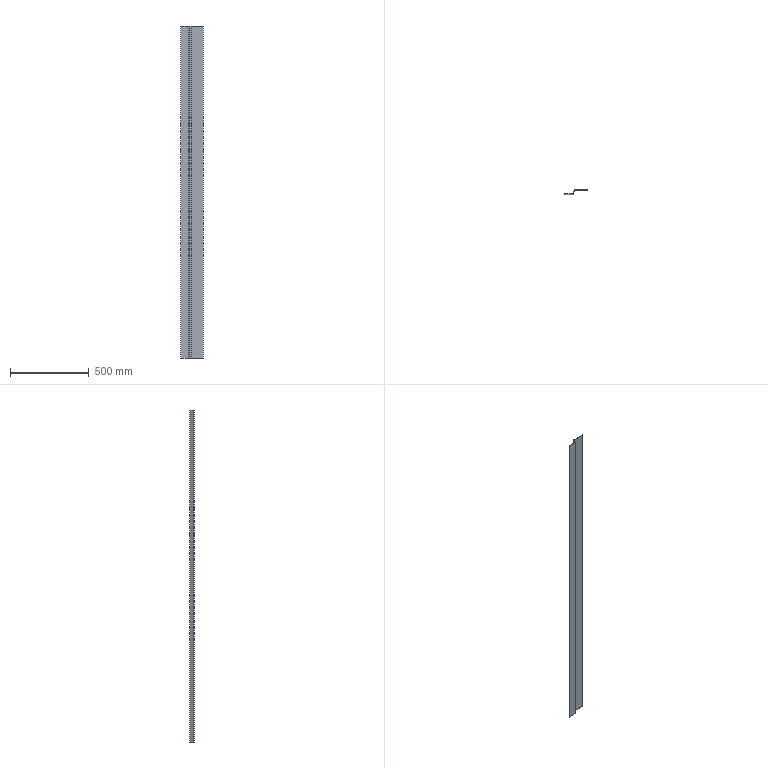Part | STEP file | 750038163 | 1 solid | 14 faces | box 144 x 29 x 2114 mm | volume 1005017 mm3 | plane 10 | cylinder 4 | commonest cylinder face diameters 6 x2 12 x2
STEP:
#1=CARTESIAN_POINT('',(-76.416,0.,1057.));
#2=VERTEX_POINT('',#1);
#3=CARTESIAN_POINT('',(0.,0.,1057.));
#4=VERTEX_POINT('',#3);
#5=CARTESIAN_POINT('',(-80.,0.,1057.));
#6=DIRECTION('',(1.,0.,0.));
#7=VECTOR('',#6,1000.);
#8=LINE('',#5,#7);
#9=EDGE_CURVE('',#2,#4,#8,.T.);
#10=ORIENTED_EDGE('',*,*,#9,.T.);
#11=CARTESIAN_POINT('',(0.,0.,-1057.));
#12=VERTEX_POINT('',#11);
#13=CARTESIAN_POINT('',(0.,0.,1057.));
#14=DIRECTION('',(0.,0.,-1.));
#15=VECTOR('',#14,1000.);
#16=LINE('',#13,#15);
#17=EDGE_CURVE('',#4,#12,#16,.T.);
#18=ORIENTED_EDGE('',*,*,#17,.T.);
#19=CARTESIAN_POINT('',(-76.416,0.,-1057.));
#20=VERTEX_POINT('',#19);
#21=CARTESIAN_POINT('',(-80.,0.,-1057.));
#22=DIRECTION('',(-1.,0.,0.));
#23=VECTOR('',#22,1000.);
#24=LINE('',#21,#23);
#25=EDGE_CURVE('',#12,#20,#24,.T.);
#26=ORIENTED_EDGE('',*,*,#25,.T.);
#27=CARTESIAN_POINT('',(-76.416,0.,1057.));
#28=DIRECTION('',(0.,0.,1.));
#29=VECTOR('',#28,1000.);
#30=LINE('',#27,#29);
#31=EDGE_CURVE('',#20,#2,#30,.T.);
#32=ORIENTED_EDGE('',*,*,#31,.T.);
#33=EDGE_LOOP('',(#10,#18,#26,#32));
#34=FACE_OUTER_BOUND('',#33,.T.);
#35=CARTESIAN_POINT('',(-80.,0.,1057.));
#36=DIRECTION('',(0.,1.,0.));
#37=DIRECTION('',(-1.,0.,0.));
#38=AXIS2_PLACEMENT_3D('',#35,#36,#37);
#39=PLANE('',#38);
#40=ADVANCED_FACE('',(#34),#39,.T.);
#41=CARTESIAN_POINT('',(0.,-3.,-1057.));
#42=VERTEX_POINT('',#41);
#43=CARTESIAN_POINT('',(0.,0.,-1057.));
#44=DIRECTION('',(0.,1.,0.));
#45=VECTOR('',#44,1000.);
#46=LINE('',#43,#45);
#47=EDGE_CURVE('',#42,#12,#46,.T.);
#48=ORIENTED_EDGE('',*,*,#47,.T.);
#49=ORIENTED_EDGE('',*,*,#17,.F.);
#50=CARTESIAN_POINT('',(0.,-3.,1057.));
#51=VERTEX_POINT('',#50);
#52=CARTESIAN_POINT('',(0.,0.,1057.));
#53=DIRECTION('',(0.,-1.,0.));
#54=VECTOR('',#53,1000.);
#55=LINE('',#52,#54);
#56=EDGE_CURVE('',#4,#51,#55,.T.);
#57=ORIENTED_EDGE('',*,*,#56,.T.);
#58=CARTESIAN_POINT('',(0.,-3.,1057.));
#59=DIRECTION('',(0.,0.,-1.));
#60=VECTOR('',#59,1000.);
#61=LINE('',#58,#60);
#62=EDGE_CURVE('',#51,#42,#61,.T.);
#63=ORIENTED_EDGE('',*,*,#62,.T.);
#64=EDGE_LOOP('',(#48,#49,#57,#63));
#65=FACE_OUTER_BOUND('',#64,.T.);
#66=CARTESIAN_POINT('',(0.,0.,1057.));
#67=DIRECTION('',(1.,0.,0.));
#68=DIRECTION('',(0.,1.,0.));
#69=AXIS2_PLACEMENT_3D('',#66,#67,#68);
#70=PLANE('',#69);
#71=ADVANCED_FACE('',(#65),#70,.T.);
#72=CARTESIAN_POINT('',(-76.416,-3.,1057.));
#73=VERTEX_POINT('',#72);
#74=CARTESIAN_POINT('',(-80.,-3.,1057.));
#75=DIRECTION('',(1.,0.,0.));
#76=VECTOR('',#75,1000.);
#77=LINE('',#74,#76);
#78=EDGE_CURVE('',#73,#51,#77,.T.);
#79=ORIENTED_EDGE('',*,*,#78,.T.);
#80=ORIENTED_EDGE('',*,*,#56,.F.);
#81=ORIENTED_EDGE('',*,*,#9,.F.);
#82=CARTESIAN_POINT('',(-81.699,-3.155,1057.));
#83=VERTEX_POINT('',#82);
#84=CARTESIAN_POINT('',(-76.416,-6.,1057.));
#85=DIRECTION('',(0.,0.,1.));
#86=DIRECTION('',(-1.,0.,0.));
#87=AXIS2_PLACEMENT_3D('',#84,#85,#86);
#88=CIRCLE('',#87,6.);
#89=EDGE_CURVE('',#2,#83,#88,.T.);
#90=ORIENTED_EDGE('',*,*,#89,.T.);
#91=CARTESIAN_POINT('',(-93.15,-24.422,1057.));
#92=VERTEX_POINT('',#91);
#93=CARTESIAN_POINT('',(-81.699,-3.155,1057.));
#94=DIRECTION('',(-0.4741,-0.8805,0.));
#95=VECTOR('',#94,1000.);
#96=LINE('',#93,#95);
#97=EDGE_CURVE('',#83,#92,#96,.T.);
#98=ORIENTED_EDGE('',*,*,#97,.T.);
#99=CARTESIAN_POINT('',(-95.792,-26.,1057.));
#100=VERTEX_POINT('',#99);
#101=CARTESIAN_POINT('',(-95.792,-23.,1057.));
#102=DIRECTION('',(0.,0.,-1.));
#103=DIRECTION('',(-1.,0.,0.));
#104=AXIS2_PLACEMENT_3D('',#101,#102,#103);
#105=CIRCLE('',#104,3.);
#106=EDGE_CURVE('',#92,#100,#105,.T.);
#107=ORIENTED_EDGE('',*,*,#106,.T.);
#108=CARTESIAN_POINT('',(-144.,-26.,1057.));
#109=VERTEX_POINT('',#108);
#110=CARTESIAN_POINT('',(-80.,-26.,1057.));
#111=DIRECTION('',(-1.,0.,0.));
#112=VECTOR('',#111,1000.);
#113=LINE('',#110,#112);
#114=EDGE_CURVE('',#100,#109,#113,.T.);
#115=ORIENTED_EDGE('',*,*,#114,.T.);
#116=CARTESIAN_POINT('',(-144.,-29.,1057.));
#117=VERTEX_POINT('',#116);
#118=CARTESIAN_POINT('',(-144.,0.,1057.));
#119=DIRECTION('',(0.,-1.,0.));
#120=VECTOR('',#119,1000.);
#121=LINE('',#118,#120);
#122=EDGE_CURVE('',#109,#117,#121,.T.);
#123=ORIENTED_EDGE('',*,*,#122,.T.);
#124=CARTESIAN_POINT('',(-95.792,-29.,1057.));
#125=VERTEX_POINT('',#124);
#126=CARTESIAN_POINT('',(-80.,-29.,1057.));
#127=DIRECTION('',(1.,0.,0.));
#128=VECTOR('',#127,1000.);
#129=LINE('',#126,#128);
#130=EDGE_CURVE('',#117,#125,#129,.T.);
#131=ORIENTED_EDGE('',*,*,#130,.T.);
#132=CARTESIAN_POINT('',(-90.509,-25.845,1057.));
#133=VERTEX_POINT('',#132);
#134=CARTESIAN_POINT('',(-95.792,-23.,1057.));
#135=DIRECTION('',(0.,0.,1.));
#136=DIRECTION('',(-1.,0.,0.));
#137=AXIS2_PLACEMENT_3D('',#134,#135,#136);
#138=CIRCLE('',#137,6.);
#139=EDGE_CURVE('',#125,#133,#138,.T.);
#140=ORIENTED_EDGE('',*,*,#139,.T.);
#141=CARTESIAN_POINT('',(-79.058,-4.578,1057.));
#142=VERTEX_POINT('',#141);
#143=CARTESIAN_POINT('',(-90.509,-25.845,1057.));
#144=DIRECTION('',(0.4741,0.8805,0.));
#145=VECTOR('',#144,1000.);
#146=LINE('',#143,#145);
#147=EDGE_CURVE('',#133,#142,#146,.T.);
#148=ORIENTED_EDGE('',*,*,#147,.T.);
#149=CARTESIAN_POINT('',(-76.416,-6.,1057.));
#150=DIRECTION('',(0.,0.,-1.));
#151=DIRECTION('',(-1.,0.,0.));
#152=AXIS2_PLACEMENT_3D('',#149,#150,#151);
#153=CIRCLE('',#152,3.);
#154=EDGE_CURVE('',#142,#73,#153,.T.);
#155=ORIENTED_EDGE('',*,*,#154,.T.);
#156=EDGE_LOOP('',(#79,#80,#81,#90,#98,#107,#115,#123,#131,#140,#148,#155));
#157=FACE_OUTER_BOUND('',#156,.T.);
#158=CARTESIAN_POINT('',(-80.,0.,1057.));
#159=DIRECTION('',(0.,0.,1.));
#160=DIRECTION('',(1.,0.,0.));
#161=AXIS2_PLACEMENT_3D('',#158,#159,#160);
#162=PLANE('',#161);
#163=ADVANCED_FACE('',(#157),#162,.T.);
#164=ORIENTED_EDGE('',*,*,#89,.F.);
#165=ORIENTED_EDGE('',*,*,#31,.F.);
#166=CARTESIAN_POINT('',(-81.699,-3.155,-1057.));
#167=VERTEX_POINT('',#166);
#168=CARTESIAN_POINT('',(-76.416,-6.,-1057.));
#169=DIRECTION('',(0.,0.,1.));
#170=DIRECTION('',(-1.,0.,0.));
#171=AXIS2_PLACEMENT_3D('',#168,#169,#170);
#172=CIRCLE('',#171,6.);
#173=EDGE_CURVE('',#20,#167,#172,.T.);
#174=ORIENTED_EDGE('',*,*,#173,.T.);
#175=CARTESIAN_POINT('',(-81.699,-3.155,1057.));
#176=DIRECTION('',(0.,0.,1.));
#177=VECTOR('',#176,1000.);
#178=LINE('',#175,#177);
#179=EDGE_CURVE('',#167,#83,#178,.T.);
#180=ORIENTED_EDGE('',*,*,#179,.T.);
#181=EDGE_LOOP('',(#164,#165,#174,#180));
#182=FACE_OUTER_BOUND('',#181,.T.);
#183=CARTESIAN_POINT('',(-76.416,-6.,1057.));
#184=DIRECTION('',(0.,0.,-1.));
#185=DIRECTION('',(-1.,0.,0.));
#186=AXIS2_PLACEMENT_3D('',#183,#184,#185);
#187=CYLINDRICAL_SURFACE('',#186,6.);
#188=ADVANCED_FACE('',(#182),#187,.T.);
#189=CARTESIAN_POINT('',(-93.15,-24.422,-1057.));
#190=VERTEX_POINT('',#189);
#191=CARTESIAN_POINT('',(-95.792,-26.,-1057.));
#192=VERTEX_POINT('',#191);
#193=CARTESIAN_POINT('',(-95.792,-23.,-1057.));
#194=DIRECTION('',(0.,0.,-1.));
#195=DIRECTION('',(-1.,0.,0.));
#196=AXIS2_PLACEMENT_3D('',#193,#194,#195);
#197=CIRCLE('',#196,3.);
#198=EDGE_CURVE('',#190,#192,#197,.T.);
#199=ORIENTED_EDGE('',*,*,#198,.F.);
#200=CARTESIAN_POINT('',(-81.699,-3.155,-1057.));
#201=DIRECTION('',(-0.4741,-0.8805,0.));
#202=VECTOR('',#201,1000.);
#203=LINE('',#200,#202);
#204=EDGE_CURVE('',#167,#190,#203,.T.);
#205=ORIENTED_EDGE('',*,*,#204,.F.);
#206=ORIENTED_EDGE('',*,*,#173,.F.);
#207=ORIENTED_EDGE('',*,*,#25,.F.);
#208=ORIENTED_EDGE('',*,*,#47,.F.);
#209=CARTESIAN_POINT('',(-76.416,-3.,-1057.));
#210=VERTEX_POINT('',#209);
#211=CARTESIAN_POINT('',(-144.,-3.,-1057.));
#212=DIRECTION('',(1.,0.,0.));
#213=VECTOR('',#212,1000.);
#214=LINE('',#211,#213);
#215=EDGE_CURVE('',#210,#42,#214,.T.);
#216=ORIENTED_EDGE('',*,*,#215,.F.);
#217=CARTESIAN_POINT('',(-79.058,-4.578,-1057.));
#218=VERTEX_POINT('',#217);
#219=CARTESIAN_POINT('',(-76.416,-6.,-1057.));
#220=DIRECTION('',(0.,0.,-1.));
#221=DIRECTION('',(-1.,0.,0.));
#222=AXIS2_PLACEMENT_3D('',#219,#220,#221);
#223=CIRCLE('',#222,3.);
#224=EDGE_CURVE('',#218,#210,#223,.T.);
#225=ORIENTED_EDGE('',*,*,#224,.F.);
#226=CARTESIAN_POINT('',(-90.509,-25.845,-1057.));
#227=VERTEX_POINT('',#226);
#228=CARTESIAN_POINT('',(-90.509,-25.845,-1057.));
#229=DIRECTION('',(0.4741,0.8805,0.));
#230=VECTOR('',#229,1000.);
#231=LINE('',#228,#230);
#232=EDGE_CURVE('',#227,#218,#231,.T.);
#233=ORIENTED_EDGE('',*,*,#232,.F.);
#234=CARTESIAN_POINT('',(-95.792,-29.,-1057.));
#235=VERTEX_POINT('',#234);
#236=CARTESIAN_POINT('',(-95.792,-23.,-1057.));
#237=DIRECTION('',(0.,0.,1.));
#238=DIRECTION('',(-1.,0.,0.));
#239=AXIS2_PLACEMENT_3D('',#236,#237,#238);
#240=CIRCLE('',#239,6.);
#241=EDGE_CURVE('',#235,#227,#240,.T.);
#242=ORIENTED_EDGE('',*,*,#241,.F.);
#243=CARTESIAN_POINT('',(-144.,-29.,-1057.));
#244=VERTEX_POINT('',#243);
#245=CARTESIAN_POINT('',(-144.,-29.,-1057.));
#246=DIRECTION('',(1.,0.,0.));
#247=VECTOR('',#246,1000.);
#248=LINE('',#245,#247);
#249=EDGE_CURVE('',#244,#235,#248,.T.);
#250=ORIENTED_EDGE('',*,*,#249,.F.);
#251=CARTESIAN_POINT('',(-144.,-26.,-1057.));
#252=VERTEX_POINT('',#251);
#253=CARTESIAN_POINT('',(-144.,-26.,-1057.));
#254=DIRECTION('',(0.,-1.,0.));
#255=VECTOR('',#254,1000.);
#256=LINE('',#253,#255);
#257=EDGE_CURVE('',#252,#244,#256,.T.);
#258=ORIENTED_EDGE('',*,*,#257,.F.);
#259=CARTESIAN_POINT('',(-144.,-26.,-1057.));
#260=DIRECTION('',(-1.,0.,0.));
#261=VECTOR('',#260,1000.);
#262=LINE('',#259,#261);
#263=EDGE_CURVE('',#192,#252,#262,.T.);
#264=ORIENTED_EDGE('',*,*,#263,.F.);
#265=EDGE_LOOP('',(#199,#205,#206,#207,#208,#216,#225,#233,#242,#250,#258,#264));
#266=FACE_OUTER_BOUND('',#265,.T.);
#267=CARTESIAN_POINT('',(-144.,-26.,-1057.));
#268=DIRECTION('',(0.,0.,1.));
#269=DIRECTION('',(1.,0.,0.));
#270=AXIS2_PLACEMENT_3D('',#267,#268,#269);
#271=PLANE('',#270);
#272=ADVANCED_FACE('',(#266),#271,.F.);
#273=ORIENTED_EDGE('',*,*,#62,.F.);
#274=ORIENTED_EDGE('',*,*,#78,.F.);
#275=CARTESIAN_POINT('',(-76.416,-3.,1057.));
#276=DIRECTION('',(0.,0.,1.));
#277=VECTOR('',#276,1000.);
#278=LINE('',#275,#277);
#279=EDGE_CURVE('',#210,#73,#278,.T.);
#280=ORIENTED_EDGE('',*,*,#279,.F.);
#281=ORIENTED_EDGE('',*,*,#215,.T.);
#282=EDGE_LOOP('',(#273,#274,#280,#281));
#283=FACE_OUTER_BOUND('',#282,.T.);
#284=CARTESIAN_POINT('',(-80.,-3.,1057.));
#285=DIRECTION('',(0.,1.,0.));
#286=DIRECTION('',(-1.,0.,0.));
#287=AXIS2_PLACEMENT_3D('',#284,#285,#286);
#288=PLANE('',#287);
#289=ADVANCED_FACE('',(#283),#288,.F.);
#290=ORIENTED_EDGE('',*,*,#279,.T.);
#291=ORIENTED_EDGE('',*,*,#154,.F.);
#292=CARTESIAN_POINT('',(-79.058,-4.578,1057.));
#293=DIRECTION('',(0.,0.,1.));
#294=VECTOR('',#293,1000.);
#295=LINE('',#292,#294);
#296=EDGE_CURVE('',#218,#142,#295,.T.);
#297=ORIENTED_EDGE('',*,*,#296,.F.);
#298=ORIENTED_EDGE('',*,*,#224,.T.);
#299=EDGE_LOOP('',(#290,#291,#297,#298));
#300=FACE_OUTER_BOUND('',#299,.T.);
#301=CARTESIAN_POINT('',(-76.416,-6.,1057.));
#302=DIRECTION('',(0.,0.,-1.));
#303=DIRECTION('',(-1.,0.,0.));
#304=AXIS2_PLACEMENT_3D('',#301,#302,#303);
#305=CYLINDRICAL_SURFACE('',#304,3.);
#306=ADVANCED_FACE('',(#300),#305,.F.);
#307=ORIENTED_EDGE('',*,*,#296,.T.);
#308=ORIENTED_EDGE('',*,*,#147,.F.);
#309=CARTESIAN_POINT('',(-90.509,-25.845,1057.));
#310=DIRECTION('',(0.,0.,1.));
#311=VECTOR('',#310,1000.);
#312=LINE('',#309,#311);
#313=EDGE_CURVE('',#227,#133,#312,.T.);
#314=ORIENTED_EDGE('',*,*,#313,.F.);
#315=ORIENTED_EDGE('',*,*,#232,.T.);
#316=EDGE_LOOP('',(#307,#308,#314,#315));
#317=FACE_OUTER_BOUND('',#316,.T.);
#318=CARTESIAN_POINT('',(-91.359,-27.422,1057.));
#319=DIRECTION('',(-0.8805,0.4741,0.));
#320=DIRECTION('',(-0.4741,-0.8805,0.));
#321=AXIS2_PLACEMENT_3D('',#318,#319,#320);
#322=PLANE('',#321);
#323=ADVANCED_FACE('',(#317),#322,.F.);
#324=ORIENTED_EDGE('',*,*,#139,.F.);
#325=CARTESIAN_POINT('',(-95.792,-29.,1057.));
#326=DIRECTION('',(0.,0.,-1.));
#327=VECTOR('',#326,1000.);
#328=LINE('',#325,#327);
#329=EDGE_CURVE('',#125,#235,#328,.T.);
#330=ORIENTED_EDGE('',*,*,#329,.T.);
#331=ORIENTED_EDGE('',*,*,#241,.T.);
#332=ORIENTED_EDGE('',*,*,#313,.T.);
#333=EDGE_LOOP('',(#324,#330,#331,#332));
#334=FACE_OUTER_BOUND('',#333,.T.);
#335=CARTESIAN_POINT('',(-95.792,-23.,1057.));
#336=DIRECTION('',(0.,0.,-1.));
#337=DIRECTION('',(-1.,0.,0.));
#338=AXIS2_PLACEMENT_3D('',#335,#336,#337);
#339=CYLINDRICAL_SURFACE('',#338,6.);
#340=ADVANCED_FACE('',(#334),#339,.T.);
#341=ORIENTED_EDGE('',*,*,#329,.F.);
#342=ORIENTED_EDGE('',*,*,#130,.F.);
#343=CARTESIAN_POINT('',(-144.,-29.,1057.));
#344=DIRECTION('',(0.,0.,1.));
#345=VECTOR('',#344,1000.);
#346=LINE('',#343,#345);
#347=EDGE_CURVE('',#244,#117,#346,.T.);
#348=ORIENTED_EDGE('',*,*,#347,.F.);
#349=ORIENTED_EDGE('',*,*,#249,.T.);
#350=EDGE_LOOP('',(#341,#342,#348,#349));
#351=FACE_OUTER_BOUND('',#350,.T.);
#352=CARTESIAN_POINT('',(-144.,-29.,1057.));
#353=DIRECTION('',(0.,1.,0.));
#354=DIRECTION('',(0.,0.,1.));
#355=AXIS2_PLACEMENT_3D('',#352,#353,#354);
#356=PLANE('',#355);
#357=ADVANCED_FACE('',(#351),#356,.F.);
#358=ORIENTED_EDGE('',*,*,#122,.F.);
#359=CARTESIAN_POINT('',(-144.,-26.,1057.));
#360=DIRECTION('',(0.,0.,1.));
#361=VECTOR('',#360,1000.);
#362=LINE('',#359,#361);
#363=EDGE_CURVE('',#252,#109,#362,.T.);
#364=ORIENTED_EDGE('',*,*,#363,.F.);
#365=ORIENTED_EDGE('',*,*,#257,.T.);
#366=ORIENTED_EDGE('',*,*,#347,.T.);
#367=EDGE_LOOP('',(#358,#364,#365,#366));
#368=FACE_OUTER_BOUND('',#367,.T.);
#369=CARTESIAN_POINT('',(-144.,-26.,1057.));
#370=DIRECTION('',(1.,0.,0.));
#371=DIRECTION('',(0.,0.,-1.));
#372=AXIS2_PLACEMENT_3D('',#369,#370,#371);
#373=PLANE('',#372);
#374=ADVANCED_FACE('',(#368),#373,.F.);
#375=ORIENTED_EDGE('',*,*,#114,.F.);
#376=CARTESIAN_POINT('',(-95.792,-26.,1057.));
#377=DIRECTION('',(0.,0.,-1.));
#378=VECTOR('',#377,1000.);
#379=LINE('',#376,#378);
#380=EDGE_CURVE('',#100,#192,#379,.T.);
#381=ORIENTED_EDGE('',*,*,#380,.T.);
#382=ORIENTED_EDGE('',*,*,#263,.T.);
#383=ORIENTED_EDGE('',*,*,#363,.T.);
#384=EDGE_LOOP('',(#375,#381,#382,#383));
#385=FACE_OUTER_BOUND('',#384,.T.);
#386=CARTESIAN_POINT('',(-144.,-26.,1057.));
#387=DIRECTION('',(0.,1.,0.));
#388=DIRECTION('',(0.,0.,1.));
#389=AXIS2_PLACEMENT_3D('',#386,#387,#388);
#390=PLANE('',#389);
#391=ADVANCED_FACE('',(#385),#390,.T.);
#392=ORIENTED_EDGE('',*,*,#380,.F.);
#393=ORIENTED_EDGE('',*,*,#106,.F.);
#394=CARTESIAN_POINT('',(-93.15,-24.422,1057.));
#395=DIRECTION('',(0.,0.,1.));
#396=VECTOR('',#395,1000.);
#397=LINE('',#394,#396);
#398=EDGE_CURVE('',#190,#92,#397,.T.);
#399=ORIENTED_EDGE('',*,*,#398,.F.);
#400=ORIENTED_EDGE('',*,*,#198,.T.);
#401=EDGE_LOOP('',(#392,#393,#399,#400));
#402=FACE_OUTER_BOUND('',#401,.T.);
#403=CARTESIAN_POINT('',(-95.792,-23.,1057.));
#404=DIRECTION('',(0.,0.,-1.));
#405=DIRECTION('',(-1.,0.,0.));
#406=AXIS2_PLACEMENT_3D('',#403,#404,#405);
#407=CYLINDRICAL_SURFACE('',#406,3.);
#408=ADVANCED_FACE('',(#402),#407,.F.);
#409=ORIENTED_EDGE('',*,*,#97,.F.);
#410=ORIENTED_EDGE('',*,*,#179,.F.);
#411=ORIENTED_EDGE('',*,*,#204,.T.);
#412=ORIENTED_EDGE('',*,*,#398,.T.);
#413=EDGE_LOOP('',(#409,#410,#411,#412));
#414=FACE_OUTER_BOUND('',#413,.T.);
#415=CARTESIAN_POINT('',(-94.,-26.,1057.));
#416=DIRECTION('',(-0.8805,0.4741,0.));
#417=DIRECTION('',(-0.4741,-0.8805,0.));
#418=AXIS2_PLACEMENT_3D('',#415,#416,#417);
#419=PLANE('',#418);
#420=ADVANCED_FACE('',(#414),#419,.T.);
#421=CLOSED_SHELL('',(#40,#71,#163,#188,#272,#289,#306,#323,#340,#357,#374,#391,#408,#420));
#422=MANIFOLD_SOLID_BREP('',#421);
#423=CARTESIAN_POINT('',(0.,0.,0.));
#424=DIRECTION('',(0.,0.,1.));
#425=DIRECTION('',(1.,0.,0.));
#426=AXIS2_PLACEMENT_3D('',#423,#424,#425);
#427=(LENGTH_UNIT()NAMED_UNIT(*)SI_UNIT(.MILLI.,.METRE.));
#428=UNCERTAINTY_MEASURE_WITH_UNIT(LENGTH_MEASURE(0.00001),#427,'','');
#429=(NAMED_UNIT(*)PLANE_ANGLE_UNIT()SI_UNIT($,.RADIAN.));
#430=(NAMED_UNIT(*)SI_UNIT($,.STERADIAN.)SOLID_ANGLE_UNIT());
#431=(GEOMETRIC_REPRESENTATION_CONTEXT(3)GLOBAL_UNCERTAINTY_ASSIGNED_CONTEXT((#428))GLOBAL_UNIT_ASSIGNED_CONTEXT((#427,#429,#430))REPRESENTATION_CONTEXT('',''));
#432=ADVANCED_BREP_SHAPE_REPRESENTATION('',(#422,#426),#431);